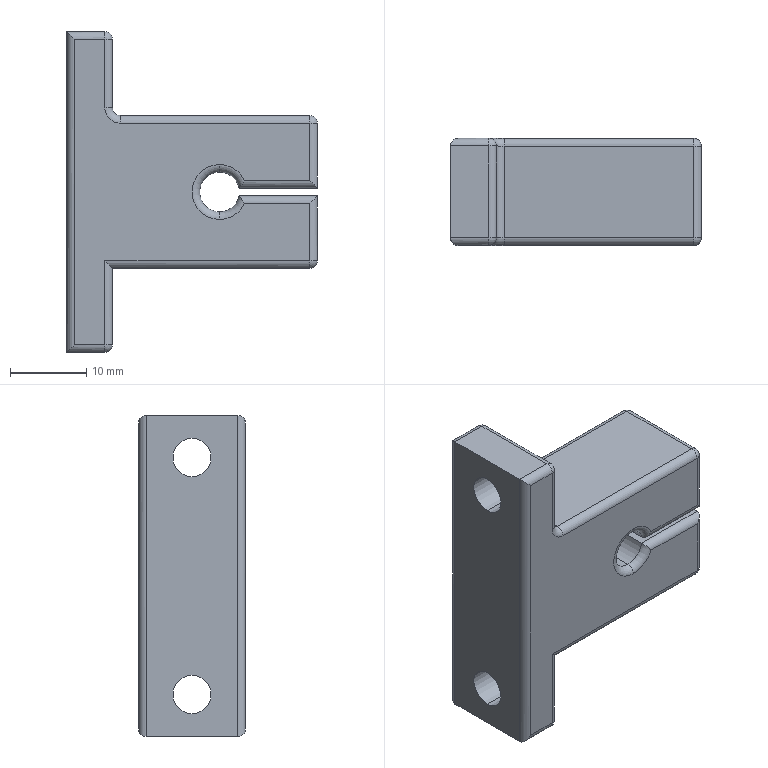Part | STEP file | T-type support 5(D) | 1 solid | 67 faces | box 32.8 x 14 x 42 mm | volume 10262 mm3 | cylinder 34 | plane 13 | torus 12 | sphere 8 | commonest cylinder face diameters 2 x27 5 x4 5.2 x3